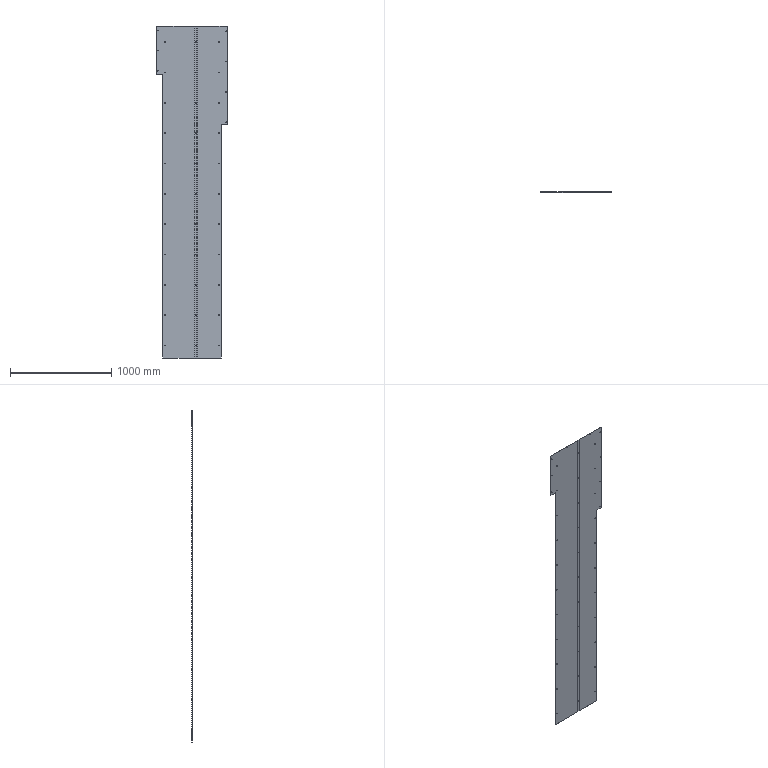Part | STEP file | TS-S31 | 1 solid | 126 faces | box 702 x 4.2 x 3283 mm | volume 2405331 mm3 | cylinder 90 | plane 36 | commonest cylinder face diameters 5.4 x80 0.4 x4 2.8 x4 10 x2